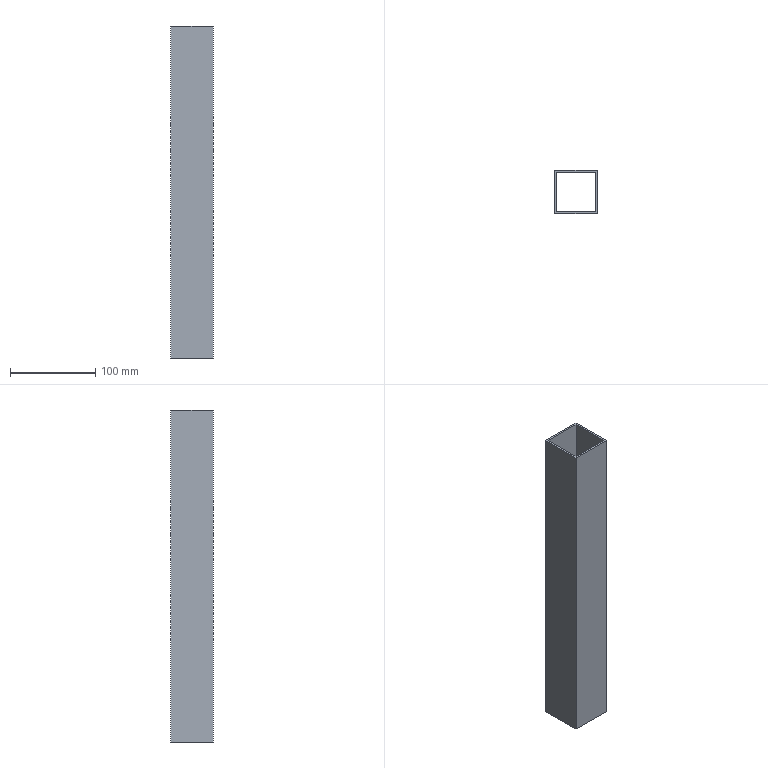Part | SolidWorks | features Extrusion 1 | 1 solid | 10 faces | box 50 x 50 x 388.8 mm | volume 149299 mm3 | plane 10
STEP:
#1=CARTESIAN_POINT('',(25.,-25.,388.8));
#2=VERTEX_POINT('',#1);
#3=CARTESIAN_POINT('',(25.,25.,388.8));
#4=VERTEX_POINT('',#3);
#5=CARTESIAN_POINT('',(25.,-25.,388.8));
#6=DIRECTION('',(0.,1.,0.));
#7=VECTOR('',#6,1000.);
#8=LINE('',#5,#7);
#9=EDGE_CURVE('',#2,#4,#8,.T.);
#10=ORIENTED_EDGE('',*,*,#9,.T.);
#11=CARTESIAN_POINT('',(-25.,25.,388.8));
#12=VERTEX_POINT('',#11);
#13=CARTESIAN_POINT('',(-25.,25.,388.8));
#14=DIRECTION('',(-1.,0.,0.));
#15=VECTOR('',#14,1000.);
#16=LINE('',#13,#15);
#17=EDGE_CURVE('',#4,#12,#16,.T.);
#18=ORIENTED_EDGE('',*,*,#17,.T.);
#19=CARTESIAN_POINT('',(-25.,-25.,388.8));
#20=VERTEX_POINT('',#19);
#21=CARTESIAN_POINT('',(-25.,-25.,388.8));
#22=DIRECTION('',(0.,-1.,0.));
#23=VECTOR('',#22,1000.);
#24=LINE('',#21,#23);
#25=EDGE_CURVE('',#12,#20,#24,.T.);
#26=ORIENTED_EDGE('',*,*,#25,.T.);
#27=CARTESIAN_POINT('',(-25.,-25.,388.8));
#28=DIRECTION('',(1.,0.,0.));
#29=VECTOR('',#28,1000.);
#30=LINE('',#27,#29);
#31=EDGE_CURVE('',#20,#2,#30,.T.);
#32=ORIENTED_EDGE('',*,*,#31,.T.);
#33=EDGE_LOOP('',(#10,#18,#26,#32));
#34=FACE_OUTER_BOUND('',#33,.T.);
#35=CARTESIAN_POINT('',(23.,-23.,388.8));
#36=VERTEX_POINT('',#35);
#37=CARTESIAN_POINT('',(23.,23.,388.8));
#38=VERTEX_POINT('',#37);
#39=CARTESIAN_POINT('',(23.,-23.,388.8));
#40=DIRECTION('',(0.,1.,0.));
#41=VECTOR('',#40,1000.);
#42=LINE('',#39,#41);
#43=EDGE_CURVE('',#36,#38,#42,.T.);
#44=ORIENTED_EDGE('',*,*,#43,.F.);
#45=CARTESIAN_POINT('',(-23.,-23.,388.8));
#46=VERTEX_POINT('',#45);
#47=CARTESIAN_POINT('',(-23.,-23.,388.8));
#48=DIRECTION('',(1.,0.,0.));
#49=VECTOR('',#48,1000.);
#50=LINE('',#47,#49);
#51=EDGE_CURVE('',#46,#36,#50,.T.);
#52=ORIENTED_EDGE('',*,*,#51,.F.);
#53=CARTESIAN_POINT('',(-23.,23.,388.8));
#54=VERTEX_POINT('',#53);
#55=CARTESIAN_POINT('',(-23.,-23.,388.8));
#56=DIRECTION('',(0.,-1.,0.));
#57=VECTOR('',#56,1000.);
#58=LINE('',#55,#57);
#59=EDGE_CURVE('',#54,#46,#58,.T.);
#60=ORIENTED_EDGE('',*,*,#59,.F.);
#61=CARTESIAN_POINT('',(-23.,23.,388.8));
#62=DIRECTION('',(-1.,0.,0.));
#63=VECTOR('',#62,1000.);
#64=LINE('',#61,#63);
#65=EDGE_CURVE('',#38,#54,#64,.T.);
#66=ORIENTED_EDGE('',*,*,#65,.F.);
#67=EDGE_LOOP('',(#44,#52,#60,#66));
#68=FACE_BOUND('',#67,.T.);
#69=CARTESIAN_POINT('',(0.,0.,388.8));
#70=DIRECTION('',(0.,0.,-1.));
#71=DIRECTION('',(-1.,0.,0.));
#72=AXIS2_PLACEMENT_3D('',#69,#70,#71);
#73=PLANE('',#72);
#74=ADVANCED_FACE('',(#34,#68),#73,.F.);
#75=CARTESIAN_POINT('',(25.,-25.,0.));
#76=VERTEX_POINT('',#75);
#77=CARTESIAN_POINT('',(25.,25.,0.));
#78=VERTEX_POINT('',#77);
#79=CARTESIAN_POINT('',(25.,-25.,0.));
#80=DIRECTION('',(0.,1.,0.));
#81=VECTOR('',#80,1000.);
#82=LINE('',#79,#81);
#83=EDGE_CURVE('',#76,#78,#82,.T.);
#84=ORIENTED_EDGE('',*,*,#83,.F.);
#85=CARTESIAN_POINT('',(-25.,-25.,0.));
#86=VERTEX_POINT('',#85);
#87=CARTESIAN_POINT('',(-25.,-25.,0.));
#88=DIRECTION('',(1.,0.,0.));
#89=VECTOR('',#88,1000.);
#90=LINE('',#87,#89);
#91=EDGE_CURVE('',#86,#76,#90,.T.);
#92=ORIENTED_EDGE('',*,*,#91,.F.);
#93=CARTESIAN_POINT('',(-25.,25.,0.));
#94=VERTEX_POINT('',#93);
#95=CARTESIAN_POINT('',(-25.,-25.,0.));
#96=DIRECTION('',(0.,-1.,0.));
#97=VECTOR('',#96,1000.);
#98=LINE('',#95,#97);
#99=EDGE_CURVE('',#94,#86,#98,.T.);
#100=ORIENTED_EDGE('',*,*,#99,.F.);
#101=CARTESIAN_POINT('',(-25.,25.,0.));
#102=DIRECTION('',(-1.,0.,0.));
#103=VECTOR('',#102,1000.);
#104=LINE('',#101,#103);
#105=EDGE_CURVE('',#78,#94,#104,.T.);
#106=ORIENTED_EDGE('',*,*,#105,.F.);
#107=EDGE_LOOP('',(#84,#92,#100,#106));
#108=FACE_OUTER_BOUND('',#107,.T.);
#109=CARTESIAN_POINT('',(-23.,-23.,0.));
#110=VERTEX_POINT('',#109);
#111=CARTESIAN_POINT('',(23.,-23.,0.));
#112=VERTEX_POINT('',#111);
#113=CARTESIAN_POINT('',(-23.,-23.,0.));
#114=DIRECTION('',(1.,0.,0.));
#115=VECTOR('',#114,1000.);
#116=LINE('',#113,#115);
#117=EDGE_CURVE('',#110,#112,#116,.T.);
#118=ORIENTED_EDGE('',*,*,#117,.T.);
#119=CARTESIAN_POINT('',(23.,23.,0.));
#120=VERTEX_POINT('',#119);
#121=CARTESIAN_POINT('',(23.,-23.,0.));
#122=DIRECTION('',(0.,1.,0.));
#123=VECTOR('',#122,1000.);
#124=LINE('',#121,#123);
#125=EDGE_CURVE('',#112,#120,#124,.T.);
#126=ORIENTED_EDGE('',*,*,#125,.T.);
#127=CARTESIAN_POINT('',(-23.,23.,0.));
#128=VERTEX_POINT('',#127);
#129=CARTESIAN_POINT('',(-23.,23.,0.));
#130=DIRECTION('',(-1.,0.,0.));
#131=VECTOR('',#130,1000.);
#132=LINE('',#129,#131);
#133=EDGE_CURVE('',#120,#128,#132,.T.);
#134=ORIENTED_EDGE('',*,*,#133,.T.);
#135=CARTESIAN_POINT('',(-23.,-23.,0.));
#136=DIRECTION('',(0.,-1.,0.));
#137=VECTOR('',#136,1000.);
#138=LINE('',#135,#137);
#139=EDGE_CURVE('',#128,#110,#138,.T.);
#140=ORIENTED_EDGE('',*,*,#139,.T.);
#141=EDGE_LOOP('',(#118,#126,#134,#140));
#142=FACE_BOUND('',#141,.T.);
#143=CARTESIAN_POINT('',(0.,0.,0.));
#144=DIRECTION('',(0.,0.,-1.));
#145=DIRECTION('',(-1.,0.,0.));
#146=AXIS2_PLACEMENT_3D('',#143,#144,#145);
#147=PLANE('',#146);
#148=ADVANCED_FACE('',(#108,#142),#147,.T.);
#149=ORIENTED_EDGE('',*,*,#83,.T.);
#150=CARTESIAN_POINT('',(25.,25.,388.8));
#151=DIRECTION('',(0.,0.,-1.));
#152=VECTOR('',#151,1000.);
#153=LINE('',#150,#152);
#154=EDGE_CURVE('',#4,#78,#153,.T.);
#155=ORIENTED_EDGE('',*,*,#154,.F.);
#156=ORIENTED_EDGE('',*,*,#9,.F.);
#157=CARTESIAN_POINT('',(25.,-25.,388.8));
#158=DIRECTION('',(0.,0.,-1.));
#159=VECTOR('',#158,1000.);
#160=LINE('',#157,#159);
#161=EDGE_CURVE('',#2,#76,#160,.T.);
#162=ORIENTED_EDGE('',*,*,#161,.T.);
#163=EDGE_LOOP('',(#149,#155,#156,#162));
#164=FACE_OUTER_BOUND('',#163,.T.);
#165=CARTESIAN_POINT('',(25.,-25.,388.8));
#166=DIRECTION('',(-1.,0.,0.));
#167=DIRECTION('',(0.,0.,1.));
#168=AXIS2_PLACEMENT_3D('',#165,#166,#167);
#169=PLANE('',#168);
#170=ADVANCED_FACE('',(#164),#169,.F.);
#171=ORIENTED_EDGE('',*,*,#105,.T.);
#172=CARTESIAN_POINT('',(-25.,25.,388.8));
#173=DIRECTION('',(0.,0.,-1.));
#174=VECTOR('',#173,1000.);
#175=LINE('',#172,#174);
#176=EDGE_CURVE('',#12,#94,#175,.T.);
#177=ORIENTED_EDGE('',*,*,#176,.F.);
#178=ORIENTED_EDGE('',*,*,#17,.F.);
#179=ORIENTED_EDGE('',*,*,#154,.T.);
#180=EDGE_LOOP('',(#171,#177,#178,#179));
#181=FACE_OUTER_BOUND('',#180,.T.);
#182=CARTESIAN_POINT('',(-25.,25.,388.8));
#183=DIRECTION('',(0.,-1.,0.));
#184=DIRECTION('',(0.,0.,-1.));
#185=AXIS2_PLACEMENT_3D('',#182,#183,#184);
#186=PLANE('',#185);
#187=ADVANCED_FACE('',(#181),#186,.F.);
#188=ORIENTED_EDGE('',*,*,#99,.T.);
#189=CARTESIAN_POINT('',(-25.,-25.,388.8));
#190=DIRECTION('',(0.,0.,-1.));
#191=VECTOR('',#190,1000.);
#192=LINE('',#189,#191);
#193=EDGE_CURVE('',#20,#86,#192,.T.);
#194=ORIENTED_EDGE('',*,*,#193,.F.);
#195=ORIENTED_EDGE('',*,*,#25,.F.);
#196=ORIENTED_EDGE('',*,*,#176,.T.);
#197=EDGE_LOOP('',(#188,#194,#195,#196));
#198=FACE_OUTER_BOUND('',#197,.T.);
#199=CARTESIAN_POINT('',(-25.,-25.,388.8));
#200=DIRECTION('',(1.,0.,0.));
#201=DIRECTION('',(0.,0.,-1.));
#202=AXIS2_PLACEMENT_3D('',#199,#200,#201);
#203=PLANE('',#202);
#204=ADVANCED_FACE('',(#198),#203,.F.);
#205=ORIENTED_EDGE('',*,*,#91,.T.);
#206=ORIENTED_EDGE('',*,*,#161,.F.);
#207=ORIENTED_EDGE('',*,*,#31,.F.);
#208=ORIENTED_EDGE('',*,*,#193,.T.);
#209=EDGE_LOOP('',(#205,#206,#207,#208));
#210=FACE_OUTER_BOUND('',#209,.T.);
#211=CARTESIAN_POINT('',(-25.,-25.,388.8));
#212=DIRECTION('',(0.,1.,0.));
#213=DIRECTION('',(0.,0.,1.));
#214=AXIS2_PLACEMENT_3D('',#211,#212,#213);
#215=PLANE('',#214);
#216=ADVANCED_FACE('',(#210),#215,.F.);
#217=ORIENTED_EDGE('',*,*,#125,.F.);
#218=CARTESIAN_POINT('',(23.,-23.,388.8));
#219=DIRECTION('',(0.,0.,-1.));
#220=VECTOR('',#219,1000.);
#221=LINE('',#218,#220);
#222=EDGE_CURVE('',#36,#112,#221,.T.);
#223=ORIENTED_EDGE('',*,*,#222,.F.);
#224=ORIENTED_EDGE('',*,*,#43,.T.);
#225=CARTESIAN_POINT('',(23.,23.,388.8));
#226=DIRECTION('',(0.,0.,-1.));
#227=VECTOR('',#226,1000.);
#228=LINE('',#225,#227);
#229=EDGE_CURVE('',#38,#120,#228,.T.);
#230=ORIENTED_EDGE('',*,*,#229,.T.);
#231=EDGE_LOOP('',(#217,#223,#224,#230));
#232=FACE_OUTER_BOUND('',#231,.T.);
#233=CARTESIAN_POINT('',(23.,-23.,388.8));
#234=DIRECTION('',(-1.,0.,0.));
#235=DIRECTION('',(0.,0.,1.));
#236=AXIS2_PLACEMENT_3D('',#233,#234,#235);
#237=PLANE('',#236);
#238=ADVANCED_FACE('',(#232),#237,.T.);
#239=ORIENTED_EDGE('',*,*,#133,.F.);
#240=ORIENTED_EDGE('',*,*,#229,.F.);
#241=ORIENTED_EDGE('',*,*,#65,.T.);
#242=CARTESIAN_POINT('',(-23.,23.,388.8));
#243=DIRECTION('',(0.,0.,-1.));
#244=VECTOR('',#243,1000.);
#245=LINE('',#242,#244);
#246=EDGE_CURVE('',#54,#128,#245,.T.);
#247=ORIENTED_EDGE('',*,*,#246,.T.);
#248=EDGE_LOOP('',(#239,#240,#241,#247));
#249=FACE_OUTER_BOUND('',#248,.T.);
#250=CARTESIAN_POINT('',(-23.,23.,388.8));
#251=DIRECTION('',(0.,-1.,0.));
#252=DIRECTION('',(0.,0.,-1.));
#253=AXIS2_PLACEMENT_3D('',#250,#251,#252);
#254=PLANE('',#253);
#255=ADVANCED_FACE('',(#249),#254,.T.);
#256=ORIENTED_EDGE('',*,*,#139,.F.);
#257=ORIENTED_EDGE('',*,*,#246,.F.);
#258=ORIENTED_EDGE('',*,*,#59,.T.);
#259=CARTESIAN_POINT('',(-23.,-23.,388.8));
#260=DIRECTION('',(0.,0.,-1.));
#261=VECTOR('',#260,1000.);
#262=LINE('',#259,#261);
#263=EDGE_CURVE('',#46,#110,#262,.T.);
#264=ORIENTED_EDGE('',*,*,#263,.T.);
#265=EDGE_LOOP('',(#256,#257,#258,#264));
#266=FACE_OUTER_BOUND('',#265,.T.);
#267=CARTESIAN_POINT('',(-23.,-23.,388.8));
#268=DIRECTION('',(1.,0.,0.));
#269=DIRECTION('',(0.,0.,-1.));
#270=AXIS2_PLACEMENT_3D('',#267,#268,#269);
#271=PLANE('',#270);
#272=ADVANCED_FACE('',(#266),#271,.T.);
#273=ORIENTED_EDGE('',*,*,#117,.F.);
#274=ORIENTED_EDGE('',*,*,#263,.F.);
#275=ORIENTED_EDGE('',*,*,#51,.T.);
#276=ORIENTED_EDGE('',*,*,#222,.T.);
#277=EDGE_LOOP('',(#273,#274,#275,#276));
#278=FACE_OUTER_BOUND('',#277,.T.);
#279=CARTESIAN_POINT('',(-23.,-23.,388.8));
#280=DIRECTION('',(0.,1.,0.));
#281=DIRECTION('',(0.,0.,1.));
#282=AXIS2_PLACEMENT_3D('',#279,#280,#281);
#283=PLANE('',#282);
#284=ADVANCED_FACE('',(#278),#283,.T.);
#285=CLOSED_SHELL('',(#74,#148,#170,#187,#204,#216,#238,#255,#272,#284));
#286=MANIFOLD_SOLID_BREP('',#285);
#287=CARTESIAN_POINT('',(0.,0.,0.));
#288=DIRECTION('',(0.,0.,1.));
#289=DIRECTION('',(1.,0.,0.));
#290=AXIS2_PLACEMENT_3D('',#287,#288,#289);
#291=(LENGTH_UNIT()NAMED_UNIT(*)SI_UNIT(.MILLI.,.METRE.));
#292=UNCERTAINTY_MEASURE_WITH_UNIT(LENGTH_MEASURE(0.00001),#291,'','');
#293=(NAMED_UNIT(*)PLANE_ANGLE_UNIT()SI_UNIT($,.RADIAN.));
#294=(NAMED_UNIT(*)SI_UNIT($,.STERADIAN.)SOLID_ANGLE_UNIT());
#295=(GEOMETRIC_REPRESENTATION_CONTEXT(3)GLOBAL_UNCERTAINTY_ASSIGNED_CONTEXT((#292))GLOBAL_UNIT_ASSIGNED_CONTEXT((#291,#293,#294))REPRESENTATION_CONTEXT('',''));
#296=ADVANCED_BREP_SHAPE_REPRESENTATION('',(#286,#290),#295);